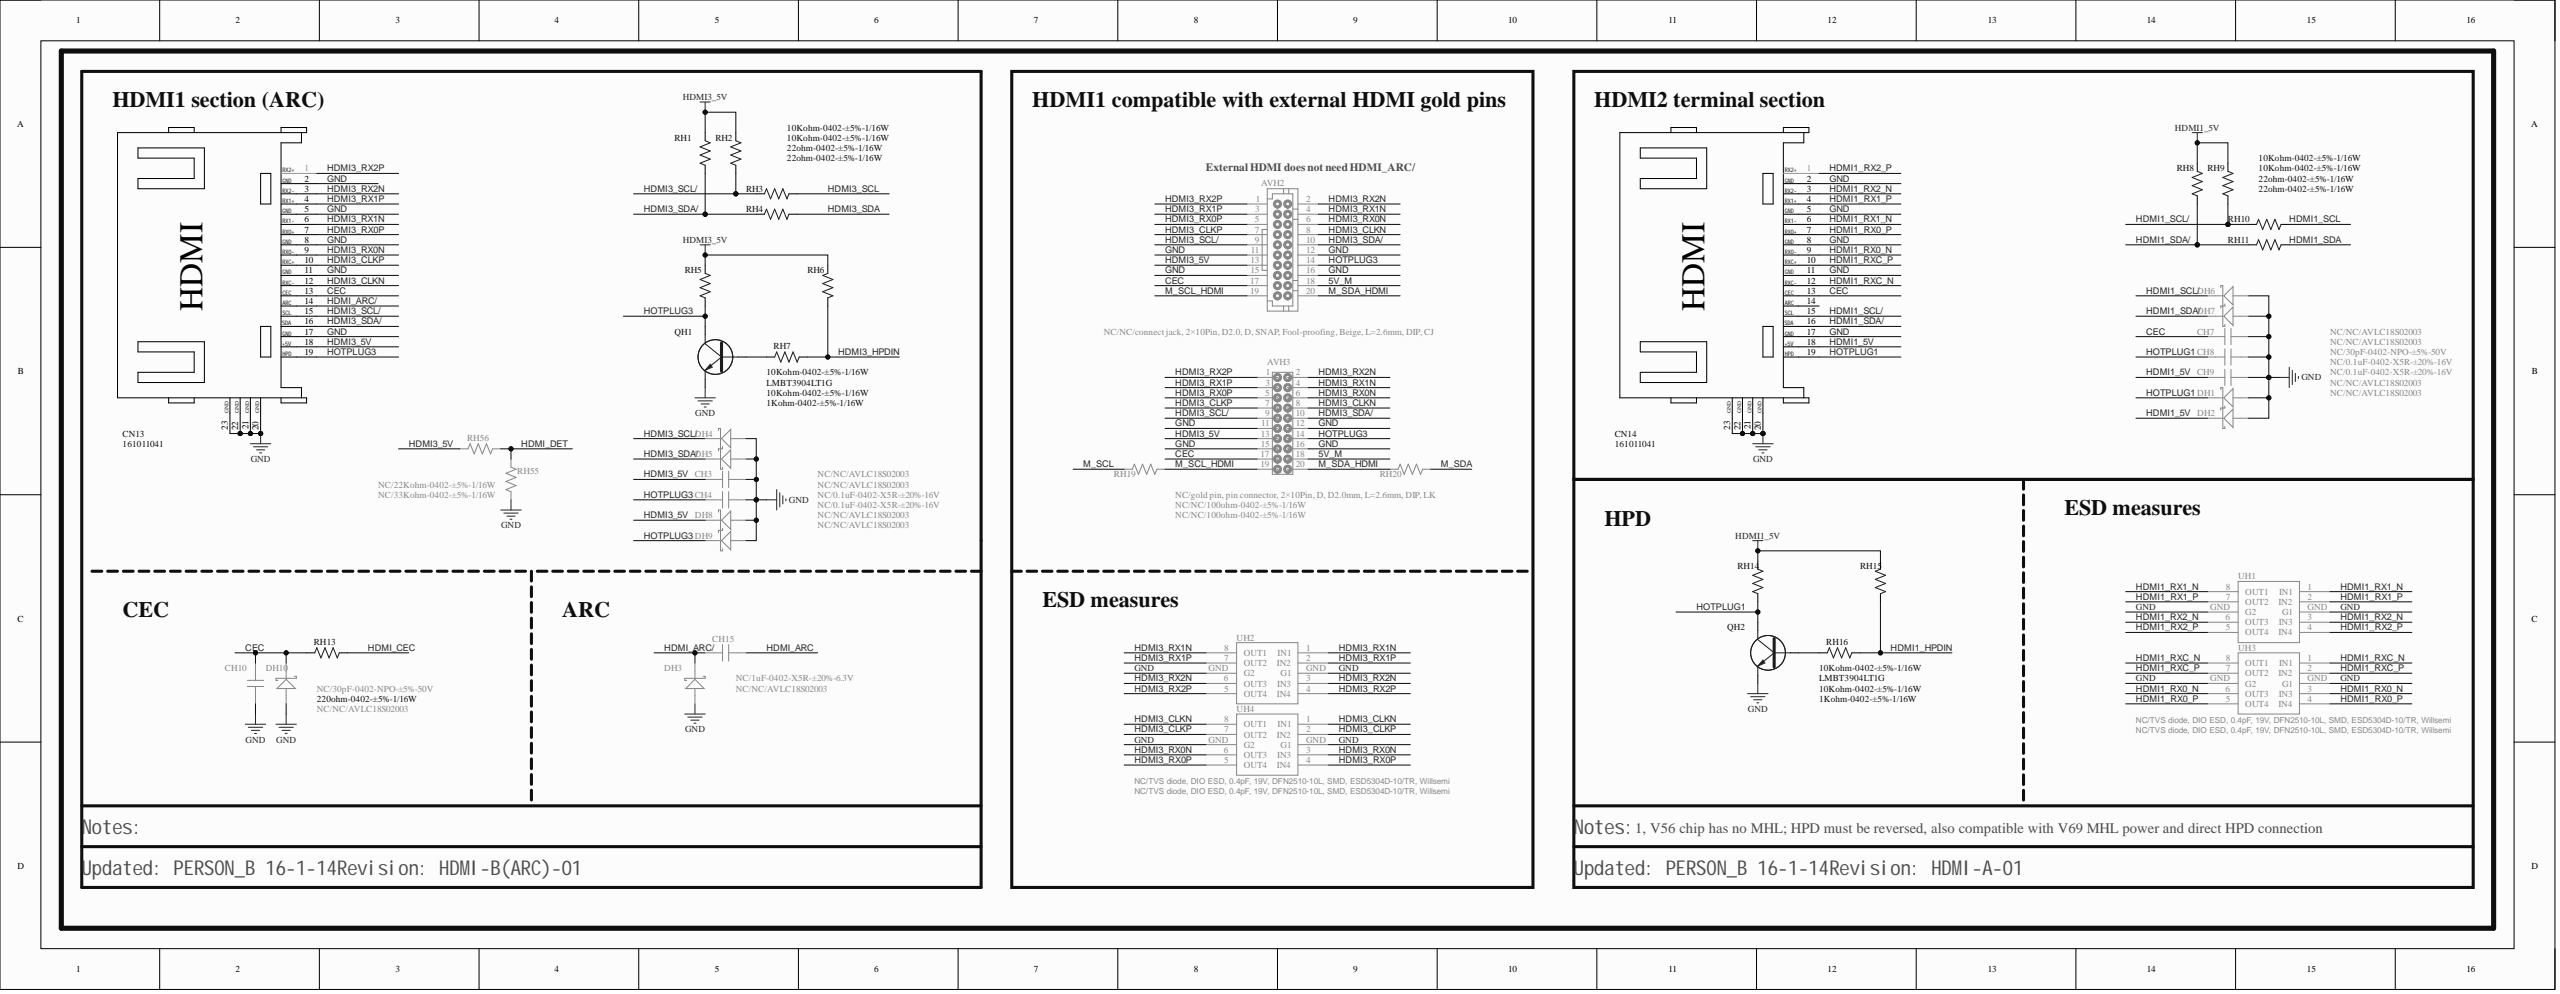Circuit board | Altium Designer | 709 parts | 378 nets | one sheet of the schematic
Parts on this sheet (reference | value | footprint):
AVH2 | NC/NC/connect jack, 2×10Pin, D2.0, D, SNAP, Fool-proofing, Beige, L=2.6mm, DIP, CJ | SIP2*10/2.0D-4
AVH3 | NC/gold pin, pin connector, 2×10Pin, D, D2.0mm, L=2.6mm, DIP, LK | SIP2*10/2.0DM-1
CH3 | NC/0.1uF-0402-X5R-±20%-16V | C0402
CH4 | NC/0.1uF-0402-X5R-±20%-16V | C0402
CH7 | NC/30pF-0402-NPO-±5%-50V | C0402
CH8 | NC/0.1uF-0402-X5R-±20%-16V | C0402
CH9 | NC/0.1uF-0402-X5R-±20%-16V | C0402
CH10 | NC/30pF-0402-NPO-±5%-50V | C0402
CH15 | NC/1uF-0402-X5R-±20%-6.3V | C0402
CN13 | 161011041 | HDMI-HS-1
CN14 | 161011041 | HDMI-HS-1
DH1 | NC/NC/AVLC18S02003 | DIODE-S0402
DH2 | NC/NC/AVLC18S02003 | DIODE-S0402
DH3 | NC/NC/AVLC18S02003 | DIODE-S0402
DH4 | NC/NC/AVLC18S02003 | DIODE-S0402
DH5 | NC/NC/AVLC18S02003 | DIODE-S0402
DH6 | NC/NC/AVLC18S02003 | DIODE-S0402
DH7 | NC/NC/AVLC18S02003 | DIODE-S0402
DH8 | NC/NC/AVLC18S02003 | DIODE-S0402
DH9 | NC/NC/AVLC18S02003 | DIODE-S0402
DH10 | NC/NC/AVLC18S02003 | DIODE-S0402
QH1 | LMBT3904LT1G | SOT-23
QH2 | LMBT3904LT1G | SOT-23
RH1 | 10Kohm-0402-±5%-1/16W | R0402
RH2 | 10Kohm-0402-±5%-1/16W | R0402
RH3 | 22ohm-0402-±5%-1/16W | R0402
RH4 | 22ohm-0402-±5%-1/16W | R0402
RH5 | 1Kohm-0402-±5%-1/16W | R0402
RH6 | 10Kohm-0402-±5%-1/16W | R0402
RH7 | 10Kohm-0402-±5%-1/16W | R0402
RH8 | 10Kohm-0402-±5%-1/16W | R0402
RH9 | 10Kohm-0402-±5%-1/16W | R0402
RH10 | 22ohm-0402-±5%-1/16W | R0402
RH11 | 22ohm-0402-±5%-1/16W | R0402
RH13 | 220ohm-0402-±5%-1/16W | R0402
RH14 | 1Kohm-0402-±5%-1/16W | R0402
RH15 | 10Kohm-0402-±5%-1/16W | R0402
RH16 | 10Kohm-0402-±5%-1/16W | R0402
RH19 | NC/NC/100ohm-0402-±5%-1/16W | R0402
RH20 | NC/NC/100ohm-0402-±5%-1/16W | R0402
RH55 | NC/33Kohm-0402-±5%-1/16W | R0402
RH56 | NC/22Kohm-0402-±5%-1/16W | R0402
UH1 | NC/TVS diode, DIO ESD, 0.4pF, 19V, DFN2510-10L, SMD, ESD5304D-10/TR, Willsemi | RCL0524P
UH2 | NC/TVS diode, DIO ESD, 0.4pF, 19V, DFN2510-10L, SMD, ESD5304D-10/TR, Willsemi | RCL0524P
UH3 | NC/TVS diode, DIO ESD, 0.4pF, 19V, DFN2510-10L, SMD, ESD5304D-10/TR, Willsemi | RCL0524P
UH4 | NC/TVS diode, DIO ESD, 0.4pF, 19V, DFN2510-10L, SMD, ESD5304D-10/TR, Willsemi | RCL0524P
Nets of these parts (net: part-pin ...):
NetQH2_B: QH2-B RH16-1
NetQH1_B: QH1-B RH7-1
M_SDA_HDMI: AVH2-20 AVH3-20 RH20-2
M_SDA: RH20-1
M_SCL_HDMI: AVH2-19 AVH3-19 RH19-2
M_SCL: RH19-1
HOTPLUG3: AVH2-14 AVH3-14 CH4-2 DH9-K QH1-C RH5-1 CN13-19
HOTPLUG1: CH8-2 DH1-K QH2-C RH14-1 CN14-19
HDMI_DET: RH55-1 RH56-1
HDMI_CEC: RH13-1
HDMI_ARC/: CH15-2 DH3-K CN13-14
HDMI_ARC: CH15-1
HDMI3_SDA/: AVH2-10 AVH3-10 DH5-K RH1-1 RH4-2 CN13-16
HDMI3_SDA: RH4-1
HDMI3_SCL/: AVH2-9 AVH3-9 DH4-K RH2-1 RH3-2 CN13-15
HDMI3_SCL: RH3-1
HDMI3_RX2P: AVH2-1 AVH3-1 UH2-4 UH2-5 CN13-1
HDMI3_RX2N: AVH2-2 AVH3-2 UH2-3 UH2-6 CN13-3
HDMI3_RX1P: AVH2-3 AVH3-3 UH2-2 UH2-7 CN13-4
HDMI3_RX1N: AVH2-4 AVH3-4 UH2-1 UH2-8 CN13-6
HDMI3_RX0P: AVH2-5 AVH3-5 UH4-4 UH4-5 CN13-7
HDMI3_RX0N: AVH2-6 AVH3-6 UH4-3 UH4-6 CN13-9
HDMI3_HPDIN: RH6-2 RH7-2
HDMI3_CLKP: AVH2-7 AVH3-7 UH4-2 UH4-7 CN13-10
HDMI3_CLKN: AVH2-8 AVH3-8 UH4-1 UH4-8 CN13-12
HDMI3_5V: AVH2-13 AVH3-13 CH3-2 DH8-K RH1-2 RH2-2 RH5-2 RH6-1 RH56-2 CN13-18
HDMI1_SDA/: DH7-K RH8-1 RH11-2 CN14-16
HDMI1_SDA: RH11-1
HDMI1_SCL/: DH6-K RH9-1 RH10-2 CN14-15
HDMI1_SCL: RH10-1
HDMI1_RXC_P: UH3-2 UH3-7 CN14-10
HDMI1_RXC_N: UH3-1 UH3-8 CN14-12
HDMI1_RX2_P: UH1-4 UH1-5 CN14-1
HDMI1_RX2_N: UH1-3 UH1-6 CN14-3
HDMI1_RX1_P: UH1-2 UH1-7 CN14-4
HDMI1_RX1_N: UH1-1 UH1-8 CN14-6
HDMI1_RX0_P: UH3-4 UH3-5 CN14-7
HDMI1_RX0_N: UH3-3 UH3-6 CN14-9
HDMI1_HPDIN: RH15-2 RH16-2
HDMI1_5V: CH9-2 DH2-K RH8-2 RH9-2 RH14-2 RH15-1 CN14-18
GND: AVH2-11 AVH2-12 AVH2-15 AVH2-16 AVH3-11 AVH3-12 AVH3-15 AVH3-16 CH3-1 CH4-1 CH7-1 CH8-1 CH9-1 CH10-1 DH1-A DH2-A DH3-A DH4-A DH5-A DH6-A DH7-A DH8-A DH9-A DH10-A QH1-E QH2-E RH55-2 UH1-GND UH2-GND UH3-GND UH4-GND CN13-2 CN13-5 CN13-8 CN13-11 CN13-17 CN13-20 CN13-21 CN13-22 CN13-23 CN14-2 CN14-5 CN14-8 CN14-11 CN14-17 CN14-20 CN14-21 CN14-22 CN14-23
CEC: AVH2-17 AVH3-17 CH7-2 CH10-2 DH10-K RH13-2 CN13-13 CN14-13
5V_M: AVH2-18 AVH3-18